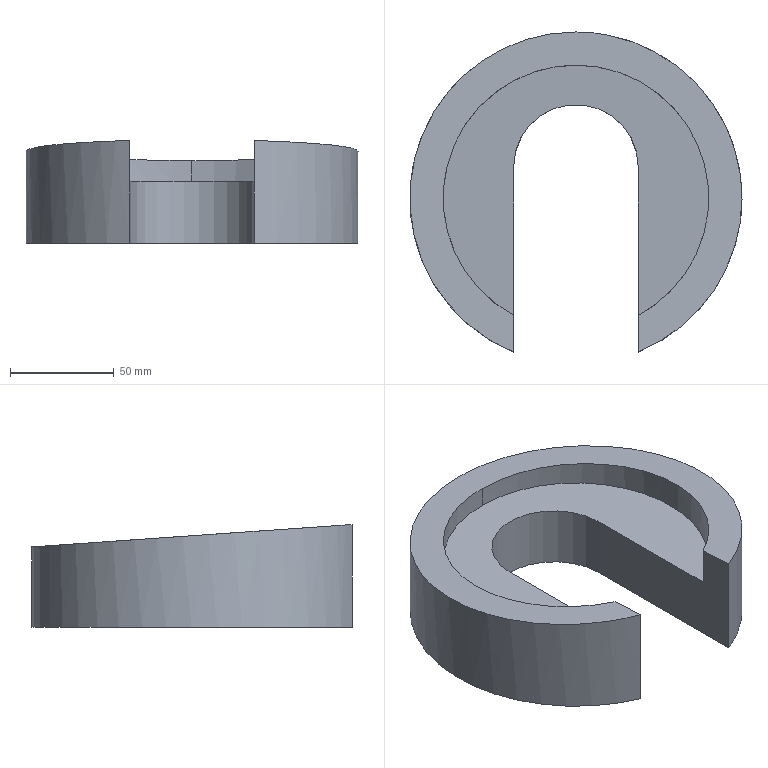Part | SolidWorks | features ICE 2, Revolution 1 | 1 solid | 10 faces | box 160 x 154.162 x 49.592 mm | volume 478394 mm3 | cylinder 5 | plane 5 | commonest cylinder face diameters 128 x2 160 x2 60 x1
STEP:
#1=CARTESIAN_POINT('',(0.,64.,39.931));
#2=VERTEX_POINT('',#1);
#3=CARTESIAN_POINT('',(30.,-56.533,48.359));
#4=VERTEX_POINT('',#3);
#5=CARTESIAN_POINT('',(0.,64.,39.931));
#6=CARTESIAN_POINT('',(83.753,64.,39.931));
#7=CARTESIAN_POINT('',(103.982,-17.274,45.614));
#8=CARTESIAN_POINT('',(30.,-56.533,48.359));
#9=(BOUNDED_CURVE()B_SPLINE_CURVE(3,(#5,#6,#7,#8),.UNSPECIFIED.,.F.,.F.)B_SPLINE_CURVE_WITH_KNOTS((4,4),(0.,2.654),.UNSPECIFIED.)CURVE()GEOMETRIC_REPRESENTATION_ITEM()RATIONAL_B_SPLINE_CURVE((1.,0.4944,0.4944,1.))REPRESENTATION_ITEM(''));
#10=EDGE_CURVE('',#2,#4,#9,.T.);
#11=ORIENTED_EDGE('',*,*,#10,.F.);
#12=CARTESIAN_POINT('',(0.,64.,30.));
#13=VERTEX_POINT('',#12);
#14=CARTESIAN_POINT('',(0.,64.,-85.977));
#15=DIRECTION('',(0.,0.,-1.));
#16=VECTOR('',#15,1000.);
#17=LINE('',#14,#16);
#18=EDGE_CURVE('',#2,#13,#17,.T.);
#19=ORIENTED_EDGE('',*,*,#18,.T.);
#20=CARTESIAN_POINT('',(30.,-56.533,30.));
#21=VERTEX_POINT('',#20);
#22=CARTESIAN_POINT('',(0.,0.,30.));
#23=DIRECTION('',(0.,0.,-1.));
#24=DIRECTION('',(0.,1.,0.));
#25=AXIS2_PLACEMENT_3D('',#22,#23,#24);
#26=CIRCLE('',#25,64.);
#27=EDGE_CURVE('',#13,#21,#26,.T.);
#28=ORIENTED_EDGE('',*,*,#27,.T.);
#29=CARTESIAN_POINT('',(30.,-56.533,-85.977));
#30=DIRECTION('',(0.,0.,1.));
#31=VECTOR('',#30,1000.);
#32=LINE('',#29,#31);
#33=EDGE_CURVE('',#21,#4,#32,.T.);
#34=ORIENTED_EDGE('',*,*,#33,.T.);
#35=EDGE_LOOP('',(#11,#19,#28,#34));
#36=FACE_OUTER_BOUND('',#35,.T.);
#37=CARTESIAN_POINT('',(0.,0.,-85.977));
#38=DIRECTION('',(0.,0.,-1.));
#39=DIRECTION('',(0.,1.,0.));
#40=AXIS2_PLACEMENT_3D('',#37,#38,#39);
#41=CYLINDRICAL_SURFACE('',#40,64.);
#42=ADVANCED_FACE('',(#36),#41,.F.);
#43=CARTESIAN_POINT('',(0.,80.,38.812));
#44=VERTEX_POINT('',#43);
#45=CARTESIAN_POINT('',(-30.,-74.162,49.592));
#46=VERTEX_POINT('',#45);
#47=CARTESIAN_POINT('',(0.,80.,38.812));
#48=CARTESIAN_POINT('',(-113.64,80.,38.812));
#49=CARTESIAN_POINT('',(-135.347,-31.547,46.612));
#50=CARTESIAN_POINT('',(-30.,-74.162,49.592));
#51=(BOUNDED_CURVE()B_SPLINE_CURVE(3,(#47,#48,#49,#50),.UNSPECIFIED.,.F.,.F.)B_SPLINE_CURVE_WITH_KNOTS((4,4),(0.,2.757),.UNSPECIFIED.)CURVE()GEOMETRIC_REPRESENTATION_ITEM()RATIONAL_B_SPLINE_CURVE((1.,0.4607,0.4607,1.))REPRESENTATION_ITEM(''));
#52=EDGE_CURVE('',#44,#46,#51,.T.);
#53=ORIENTED_EDGE('',*,*,#52,.F.);
#54=CARTESIAN_POINT('',(0.,80.,0.));
#55=VERTEX_POINT('',#54);
#56=CARTESIAN_POINT('',(0.,80.,-85.977));
#57=DIRECTION('',(0.,0.,-1.));
#58=VECTOR('',#57,1000.);
#59=LINE('',#56,#58);
#60=EDGE_CURVE('',#44,#55,#59,.T.);
#61=ORIENTED_EDGE('',*,*,#60,.T.);
#62=CARTESIAN_POINT('',(-30.,-74.162,0.));
#63=VERTEX_POINT('',#62);
#64=CARTESIAN_POINT('',(0.,0.,0.));
#65=DIRECTION('',(0.,0.,-1.));
#66=DIRECTION('',(0.,1.,0.));
#67=AXIS2_PLACEMENT_3D('',#64,#65,#66);
#68=CIRCLE('',#67,80.);
#69=EDGE_CURVE('',#63,#55,#68,.T.);
#70=ORIENTED_EDGE('',*,*,#69,.F.);
#71=CARTESIAN_POINT('',(-30.,-74.162,-85.977));
#72=DIRECTION('',(0.,0.,1.));
#73=VECTOR('',#72,1000.);
#74=LINE('',#71,#73);
#75=EDGE_CURVE('',#63,#46,#74,.T.);
#76=ORIENTED_EDGE('',*,*,#75,.T.);
#77=EDGE_LOOP('',(#53,#61,#70,#76));
#78=FACE_OUTER_BOUND('',#77,.T.);
#79=CARTESIAN_POINT('',(0.,0.,-85.977));
#80=DIRECTION('',(0.,0.,-1.));
#81=DIRECTION('',(0.,1.,0.));
#82=AXIS2_PLACEMENT_3D('',#79,#80,#81);
#83=CYLINDRICAL_SURFACE('',#82,80.);
#84=ADVANCED_FACE('',(#78),#83,.T.);
#85=CARTESIAN_POINT('',(30.,15.,0.));
#86=VERTEX_POINT('',#85);
#87=CARTESIAN_POINT('',(-30.,15.,0.));
#88=VERTEX_POINT('',#87);
#89=CARTESIAN_POINT('',(0.,15.,0.));
#90=DIRECTION('',(0.,0.,1.));
#91=DIRECTION('',(1.,0.,0.));
#92=AXIS2_PLACEMENT_3D('',#89,#90,#91);
#93=CIRCLE('',#92,30.);
#94=EDGE_CURVE('',#86,#88,#93,.T.);
#95=ORIENTED_EDGE('',*,*,#94,.T.);
#96=CARTESIAN_POINT('',(-30.,15.,0.));
#97=DIRECTION('',(0.,-1.,0.));
#98=VECTOR('',#97,1000.);
#99=LINE('',#96,#98);
#100=EDGE_CURVE('',#88,#63,#99,.T.);
#101=ORIENTED_EDGE('',*,*,#100,.T.);
#102=ORIENTED_EDGE('',*,*,#69,.T.);
#103=CARTESIAN_POINT('',(30.,-74.162,0.));
#104=VERTEX_POINT('',#103);
#105=CARTESIAN_POINT('',(0.,0.,0.));
#106=DIRECTION('',(0.,0.,-1.));
#107=DIRECTION('',(0.,1.,0.));
#108=AXIS2_PLACEMENT_3D('',#105,#106,#107);
#109=CIRCLE('',#108,80.);
#110=EDGE_CURVE('',#55,#104,#109,.T.);
#111=ORIENTED_EDGE('',*,*,#110,.T.);
#112=CARTESIAN_POINT('',(30.,15.,0.));
#113=DIRECTION('',(0.,1.,0.));
#114=VECTOR('',#113,1000.);
#115=LINE('',#112,#114);
#116=EDGE_CURVE('',#104,#86,#115,.T.);
#117=ORIENTED_EDGE('',*,*,#116,.T.);
#118=EDGE_LOOP('',(#95,#101,#102,#111,#117));
#119=FACE_OUTER_BOUND('',#118,.T.);
#120=CARTESIAN_POINT('',(0.,80.,0.));
#121=DIRECTION('',(0.,0.,-1.));
#122=DIRECTION('',(0.,1.,0.));
#123=AXIS2_PLACEMENT_3D('',#120,#121,#122);
#124=PLANE('',#123);
#125=ADVANCED_FACE('',(#119),#124,.T.);
#126=ORIENTED_EDGE('',*,*,#60,.F.);
#127=CARTESIAN_POINT('',(30.,-74.162,49.592));
#128=VERTEX_POINT('',#127);
#129=CARTESIAN_POINT('',(30.,-74.162,49.592));
#130=CARTESIAN_POINT('',(135.347,-31.547,46.612));
#131=CARTESIAN_POINT('',(113.64,80.,38.812));
#132=CARTESIAN_POINT('',(0.,80.,38.812));
#133=(BOUNDED_CURVE()B_SPLINE_CURVE(3,(#129,#130,#131,#132),.UNSPECIFIED.,.F.,.F.)B_SPLINE_CURVE_WITH_KNOTS((4,4),(3.526,6.283),.UNSPECIFIED.)CURVE()GEOMETRIC_REPRESENTATION_ITEM()RATIONAL_B_SPLINE_CURVE((1.,0.4607,0.4607,1.))REPRESENTATION_ITEM(''));
#134=EDGE_CURVE('',#128,#44,#133,.T.);
#135=ORIENTED_EDGE('',*,*,#134,.F.);
#136=CARTESIAN_POINT('',(30.,-74.162,-85.977));
#137=DIRECTION('',(0.,0.,-1.));
#138=VECTOR('',#137,1000.);
#139=LINE('',#136,#138);
#140=EDGE_CURVE('',#128,#104,#139,.T.);
#141=ORIENTED_EDGE('',*,*,#140,.T.);
#142=ORIENTED_EDGE('',*,*,#110,.F.);
#143=EDGE_LOOP('',(#126,#135,#141,#142));
#144=FACE_OUTER_BOUND('',#143,.T.);
#145=CARTESIAN_POINT('',(0.,0.,-85.977));
#146=DIRECTION('',(0.,0.,-1.));
#147=DIRECTION('',(0.,1.,0.));
#148=AXIS2_PLACEMENT_3D('',#145,#146,#147);
#149=CYLINDRICAL_SURFACE('',#148,80.);
#150=ADVANCED_FACE('',(#144),#149,.T.);
#151=CARTESIAN_POINT('',(-30.,-56.533,48.359));
#152=VERTEX_POINT('',#151);
#153=CARTESIAN_POINT('',(-30.,80.,38.812));
#154=DIRECTION('',(0.,-0.9976,0.06976));
#155=VECTOR('',#154,1000.);
#156=LINE('',#153,#155);
#157=EDGE_CURVE('',#152,#46,#156,.T.);
#158=ORIENTED_EDGE('',*,*,#157,.F.);
#159=CARTESIAN_POINT('',(-30.,-56.533,48.359));
#160=CARTESIAN_POINT('',(-103.982,-17.274,45.614));
#161=CARTESIAN_POINT('',(-83.753,64.,39.931));
#162=CARTESIAN_POINT('',(0.,64.,39.931));
#163=(BOUNDED_CURVE()B_SPLINE_CURVE(3,(#159,#160,#161,#162),.UNSPECIFIED.,.F.,.F.)B_SPLINE_CURVE_WITH_KNOTS((4,4),(3.629,6.283),.UNSPECIFIED.)CURVE()GEOMETRIC_REPRESENTATION_ITEM()RATIONAL_B_SPLINE_CURVE((1.,0.4944,0.4944,1.))REPRESENTATION_ITEM(''));
#164=EDGE_CURVE('',#152,#2,#163,.T.);
#165=ORIENTED_EDGE('',*,*,#164,.T.);
#166=ORIENTED_EDGE('',*,*,#10,.T.);
#167=CARTESIAN_POINT('',(30.,80.,38.812));
#168=DIRECTION('',(0.,0.9976,-0.06976));
#169=VECTOR('',#168,1000.);
#170=LINE('',#167,#169);
#171=EDGE_CURVE('',#128,#4,#170,.T.);
#172=ORIENTED_EDGE('',*,*,#171,.F.);
#173=ORIENTED_EDGE('',*,*,#134,.T.);
#174=ORIENTED_EDGE('',*,*,#52,.T.);
#175=EDGE_LOOP('',(#158,#165,#166,#172,#173,#174));
#176=FACE_OUTER_BOUND('',#175,.T.);
#177=CARTESIAN_POINT('',(-80.,80.,38.812));
#178=DIRECTION('',(0.,-0.06976,-0.9976));
#179=DIRECTION('',(0.,0.9976,-0.06976));
#180=AXIS2_PLACEMENT_3D('',#177,#178,#179);
#181=PLANE('',#180);
#182=ADVANCED_FACE('',(#176),#181,.F.);
#183=CARTESIAN_POINT('',(-30.,-56.533,30.));
#184=VERTEX_POINT('',#183);
#185=CARTESIAN_POINT('',(0.,0.,30.));
#186=DIRECTION('',(0.,0.,-1.));
#187=DIRECTION('',(0.,1.,0.));
#188=AXIS2_PLACEMENT_3D('',#185,#186,#187);
#189=CIRCLE('',#188,64.);
#190=EDGE_CURVE('',#184,#13,#189,.T.);
#191=ORIENTED_EDGE('',*,*,#190,.F.);
#192=CARTESIAN_POINT('',(-30.,15.,30.));
#193=VERTEX_POINT('',#192);
#194=CARTESIAN_POINT('',(-30.,64.,30.));
#195=DIRECTION('',(0.,1.,0.));
#196=VECTOR('',#195,1000.);
#197=LINE('',#194,#196);
#198=EDGE_CURVE('',#184,#193,#197,.T.);
#199=ORIENTED_EDGE('',*,*,#198,.T.);
#200=CARTESIAN_POINT('',(30.,15.,30.));
#201=VERTEX_POINT('',#200);
#202=CARTESIAN_POINT('',(0.,15.,30.));
#203=DIRECTION('',(0.,0.,-1.));
#204=DIRECTION('',(0.,-1.,0.));
#205=AXIS2_PLACEMENT_3D('',#202,#203,#204);
#206=CIRCLE('',#205,30.);
#207=EDGE_CURVE('',#193,#201,#206,.T.);
#208=ORIENTED_EDGE('',*,*,#207,.T.);
#209=CARTESIAN_POINT('',(30.,64.,30.));
#210=DIRECTION('',(0.,-1.,0.));
#211=VECTOR('',#210,1000.);
#212=LINE('',#209,#211);
#213=EDGE_CURVE('',#201,#21,#212,.T.);
#214=ORIENTED_EDGE('',*,*,#213,.T.);
#215=ORIENTED_EDGE('',*,*,#27,.F.);
#216=EDGE_LOOP('',(#191,#199,#208,#214,#215));
#217=FACE_OUTER_BOUND('',#216,.T.);
#218=CARTESIAN_POINT('',(0.,64.,30.));
#219=DIRECTION('',(0.,0.,1.));
#220=DIRECTION('',(0.,-1.,0.));
#221=AXIS2_PLACEMENT_3D('',#218,#219,#220);
#222=PLANE('',#221);
#223=ADVANCED_FACE('',(#217),#222,.T.);
#224=ORIENTED_EDGE('',*,*,#18,.F.);
#225=ORIENTED_EDGE('',*,*,#164,.F.);
#226=CARTESIAN_POINT('',(-30.,-56.533,-85.977));
#227=DIRECTION('',(0.,0.,-1.));
#228=VECTOR('',#227,1000.);
#229=LINE('',#226,#228);
#230=EDGE_CURVE('',#152,#184,#229,.T.);
#231=ORIENTED_EDGE('',*,*,#230,.T.);
#232=ORIENTED_EDGE('',*,*,#190,.T.);
#233=EDGE_LOOP('',(#224,#225,#231,#232));
#234=FACE_OUTER_BOUND('',#233,.T.);
#235=CARTESIAN_POINT('',(0.,0.,-85.977));
#236=DIRECTION('',(0.,0.,-1.));
#237=DIRECTION('',(0.,1.,0.));
#238=AXIS2_PLACEMENT_3D('',#235,#236,#237);
#239=CYLINDRICAL_SURFACE('',#238,64.);
#240=ADVANCED_FACE('',(#234),#239,.F.);
#241=CARTESIAN_POINT('',(-30.,15.,50.));
#242=DIRECTION('',(0.,0.,-1.));
#243=VECTOR('',#242,1000.);
#244=LINE('',#241,#243);
#245=EDGE_CURVE('',#193,#88,#244,.T.);
#246=ORIENTED_EDGE('',*,*,#245,.T.);
#247=ORIENTED_EDGE('',*,*,#94,.F.);
#248=CARTESIAN_POINT('',(30.,15.,50.));
#249=DIRECTION('',(0.,0.,-1.));
#250=VECTOR('',#249,1000.);
#251=LINE('',#248,#250);
#252=EDGE_CURVE('',#201,#86,#251,.T.);
#253=ORIENTED_EDGE('',*,*,#252,.F.);
#254=ORIENTED_EDGE('',*,*,#207,.F.);
#255=EDGE_LOOP('',(#246,#247,#253,#254));
#256=FACE_OUTER_BOUND('',#255,.T.);
#257=CARTESIAN_POINT('',(0.,15.,50.));
#258=DIRECTION('',(0.,0.,-1.));
#259=DIRECTION('',(-1.,0.,0.));
#260=AXIS2_PLACEMENT_3D('',#257,#258,#259);
#261=CYLINDRICAL_SURFACE('',#260,30.);
#262=ADVANCED_FACE('',(#256),#261,.F.);
#263=ORIENTED_EDGE('',*,*,#100,.F.);
#264=ORIENTED_EDGE('',*,*,#245,.F.);
#265=ORIENTED_EDGE('',*,*,#198,.F.);
#266=ORIENTED_EDGE('',*,*,#230,.F.);
#267=ORIENTED_EDGE('',*,*,#157,.T.);
#268=ORIENTED_EDGE('',*,*,#75,.F.);
#269=EDGE_LOOP('',(#263,#264,#265,#266,#267,#268));
#270=FACE_OUTER_BOUND('',#269,.T.);
#271=CARTESIAN_POINT('',(-30.,15.,50.));
#272=DIRECTION('',(1.,0.,0.));
#273=DIRECTION('',(0.,1.,0.));
#274=AXIS2_PLACEMENT_3D('',#271,#272,#273);
#275=PLANE('',#274);
#276=ADVANCED_FACE('',(#270),#275,.T.);
#277=ORIENTED_EDGE('',*,*,#171,.T.);
#278=ORIENTED_EDGE('',*,*,#33,.F.);
#279=ORIENTED_EDGE('',*,*,#213,.F.);
#280=ORIENTED_EDGE('',*,*,#252,.T.);
#281=ORIENTED_EDGE('',*,*,#116,.F.);
#282=ORIENTED_EDGE('',*,*,#140,.F.);
#283=EDGE_LOOP('',(#277,#278,#279,#280,#281,#282));
#284=FACE_OUTER_BOUND('',#283,.T.);
#285=CARTESIAN_POINT('',(30.,15.,50.));
#286=DIRECTION('',(-1.,0.,0.));
#287=DIRECTION('',(0.,-1.,0.));
#288=AXIS2_PLACEMENT_3D('',#285,#286,#287);
#289=PLANE('',#288);
#290=ADVANCED_FACE('',(#284),#289,.T.);
#291=CLOSED_SHELL('',(#42,#84,#125,#150,#182,#223,#240,#262,#276,#290));
#292=MANIFOLD_SOLID_BREP('',#291);
#293=CARTESIAN_POINT('',(0.,0.,0.));
#294=DIRECTION('',(0.,0.,1.));
#295=DIRECTION('',(1.,0.,0.));
#296=AXIS2_PLACEMENT_3D('',#293,#294,#295);
#297=(LENGTH_UNIT()NAMED_UNIT(*)SI_UNIT(.MILLI.,.METRE.));
#298=UNCERTAINTY_MEASURE_WITH_UNIT(LENGTH_MEASURE(0.00001),#297,'','');
#299=(NAMED_UNIT(*)PLANE_ANGLE_UNIT()SI_UNIT($,.RADIAN.));
#300=(NAMED_UNIT(*)SI_UNIT($,.STERADIAN.)SOLID_ANGLE_UNIT());
#301=(GEOMETRIC_REPRESENTATION_CONTEXT(3)GLOBAL_UNCERTAINTY_ASSIGNED_CONTEXT((#298))GLOBAL_UNIT_ASSIGNED_CONTEXT((#297,#299,#300))REPRESENTATION_CONTEXT('',''));
#302=ADVANCED_BREP_SHAPE_REPRESENTATION('',(#292,#296),#301);